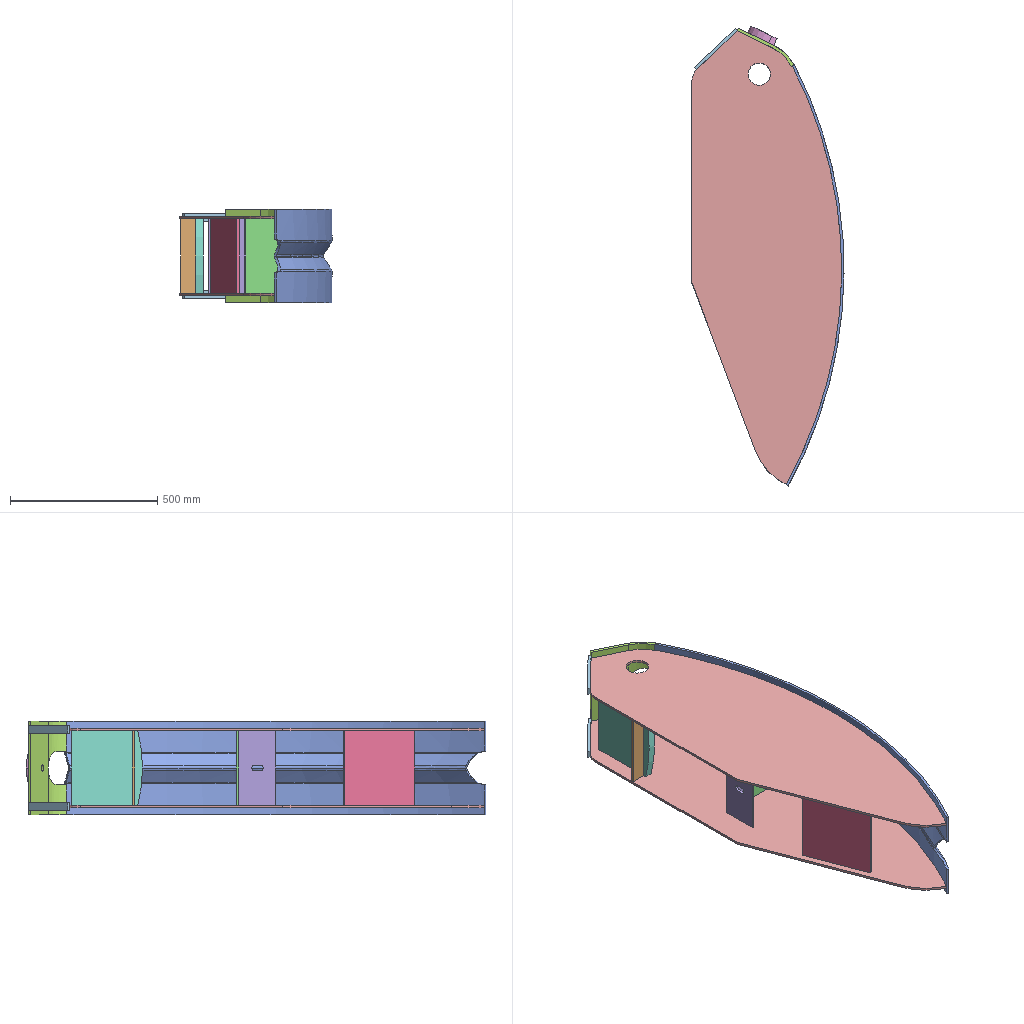Assembly | SolidWorks | 10 different items | 12 placed | box 516 x 1561 x 318 mm
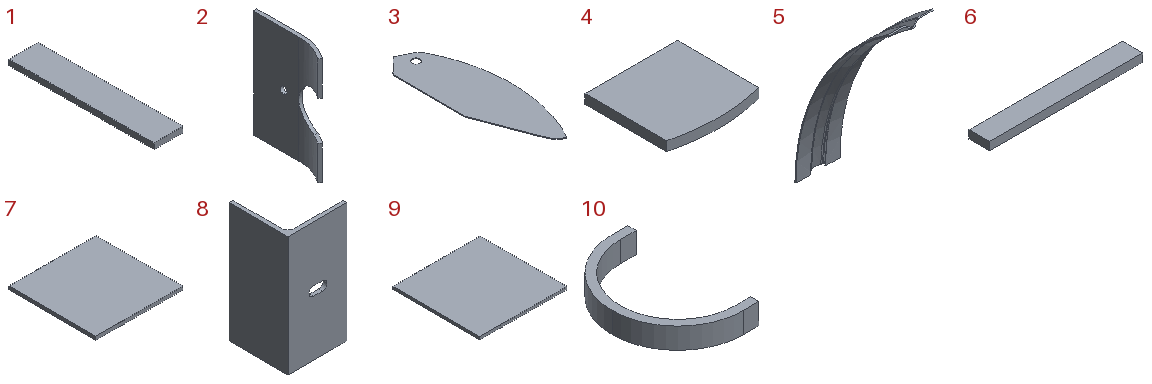Parts list (item | quantity | size | volume | features):
1 | x1 | 50.8 x 254 x 10 mm | 129032 mm3 | features Extrusion 1
2 | x1 | 38.131 x 223.442 x 317.5 mm | 624053 mm3 | features Extrusion 1, ICE 1
3 | x2 | 508 x 1540 x 8 mm | 4517145 mm3 | features Extrusion 1
4 | x1 | 254 x 241.3 x 26 mm | 1558264 mm3 | features Extrusion 1
5 | x1 | 317.5 x 695.606 x 1261 mm | 3914320 mm3 | features ICE 1, Sweep 1
6 | x2 | 190.5 x 25.4 x 10 mm | 48387 mm3 | features Extrusion 1
7 | x1 | 254 x 254 x 10 mm | 645160 mm3 | features Extrusion 1
8 | x1 | 125 x 125 x 254 mm | 495500 mm3 | features Extrusion 1, ICE 1
9 | x1 | 254 x 254 x 8 mm | 516128 mm3 | features Extrusion 1
10 | x1 | 98.425 x 158.75 x 25.4 mm | 69026 mm3 | features Extrusion 1
Mates (type | each side: item.copy, entity, surface, feature):
Coincident | 3.1 plane | assembly plane | 2 times
Coincident | 3.1 plane | 3.2 plane | 2 times
DistanceDim | 3.1 face plane Boss-Extrude1 | 3.2 face plane Boss-Extrude1
Symmetric | 3.1 face plane Boss-Extrude1 | 3.2 face plane Boss-Extrude1 | assembly plane
Concentric | 3.1 face cylinder Boss-Extrude1 | 5.1 face cylinder Sweep1
Coincident | 5.1 plane | assembly plane
Coincident | 2.1 plane | assembly plane
Coincident | 3.1 face plane Boss-Extrude1 | 2.1 face plane Boss-Extrude1
Coincident | 3.1 edge | 2.1 face plane Boss-Extrude1
Coincident | 3.1 edge | 5.1 face plane Sweep1
Coincident | 2.1 face plane Boss-Extrude1 | 10.1 face plane Boss-Extrude1
Coincident | 10.1 plane | assembly plane
Coincident | 2.1 edge | 10.1 face plane Boss-Extrude1
Coincident | 4.1 plane | assembly plane
DistanceDim | 4.1 face plane Boss-Extrude1 | 3.2 face plane Boss-Extrude1
DistanceDim | 4.1 face plane Boss-Extrude1 | assembly plane
Coincident | 1.1 plane | assembly plane
Coincident | 4.1 face plane Boss-Extrude1 | 1.1 face plane Boss-Extrude1
DistanceDim | 1.1 face plane Boss-Extrude1 | 4.1 face plane Boss-Extrude1
Coincident | 8.1 plane | assembly plane
DistanceDim | 8.1 face plane Boss-Extrude1 | 4.1 face plane Boss-Extrude1 | 2 times
Coincident | 9.1 plane | assembly plane
Coincident | 8.1 face plane Boss-Extrude1 | 9.1 face plane Boss-Extrude1
DistanceDim | 8.1 face plane Boss-Extrude1 | 9.1 face plane Boss-Extrude1
Coincident | 7.1 plane | assembly plane
DistanceDim | 7.1 face plane Boss-Extrude1 | 3.2 face plane Boss-Extrude1
DistanceDim | 7.1 edge | assembly plane
Coincident | 3.2 face plane Boss-Extrude1 | 6.1 face plane Boss-Extrude1
Coincident | 3.2 edge | 6.1 face plane Boss-Extrude1
Coincident | 3.2 plane | 6.1 plane